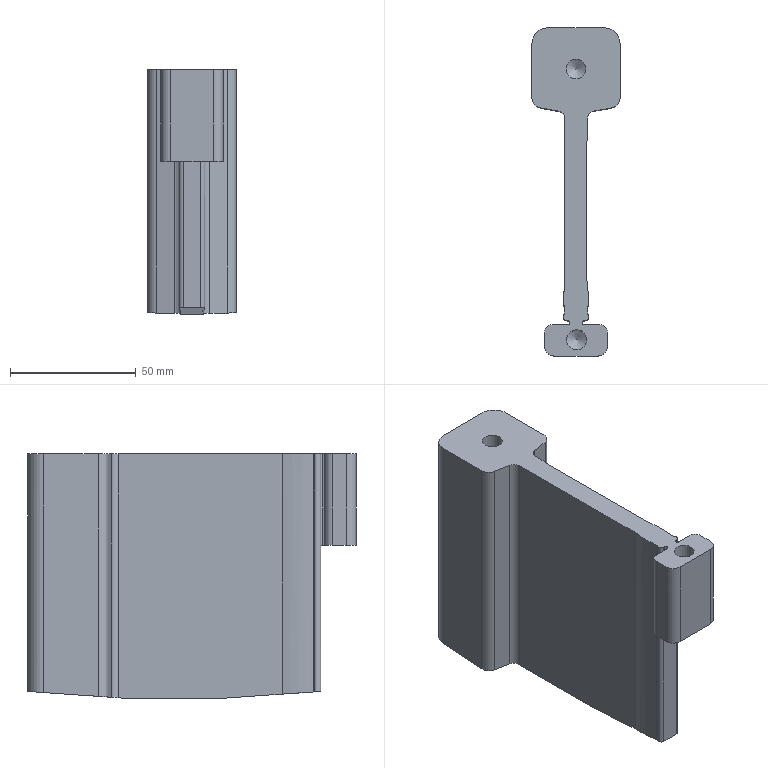Part | STEP file | 1_id142_x_t | 1 solid | 44 faces | box 35 x 130.5 x 97.111 mm | volume 188320 mm3 | cylinder 23 | plane 19 | cone 2 | commonest cylinder face diameters 1.5 x4 3 x4 6 x4 8 x4 7.938 x2 12.7 x2